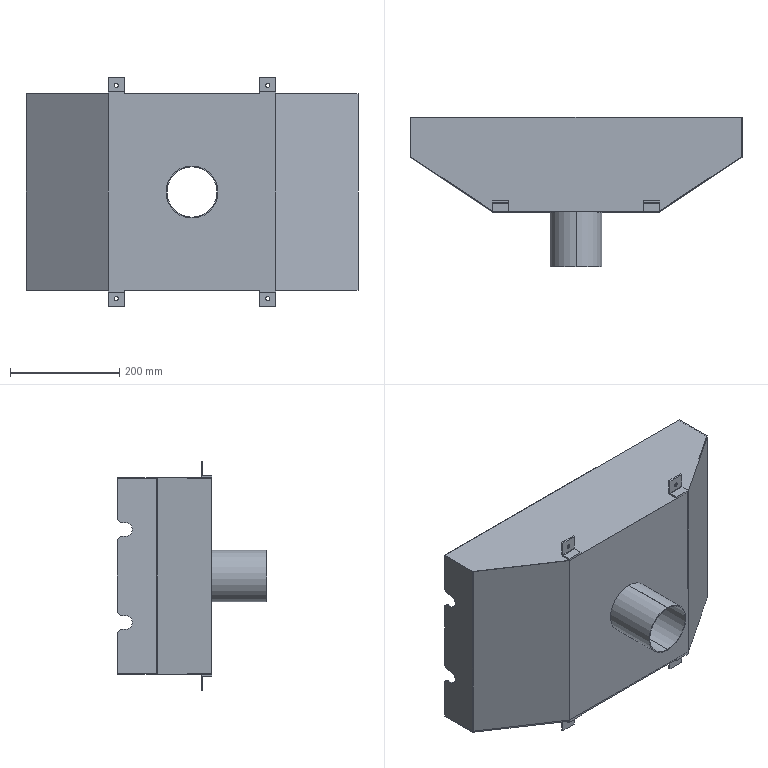Part | SolidWorks | features BaseBody 1 | 1 solid | 83 faces | box 607 x 273 x 420 mm | volume 750527 mm3 | plane 51 | cylinder 32 | commonest cylinder face diameters 7 x8 20 x8 2 x4 8 x4 25 x4 92 x2